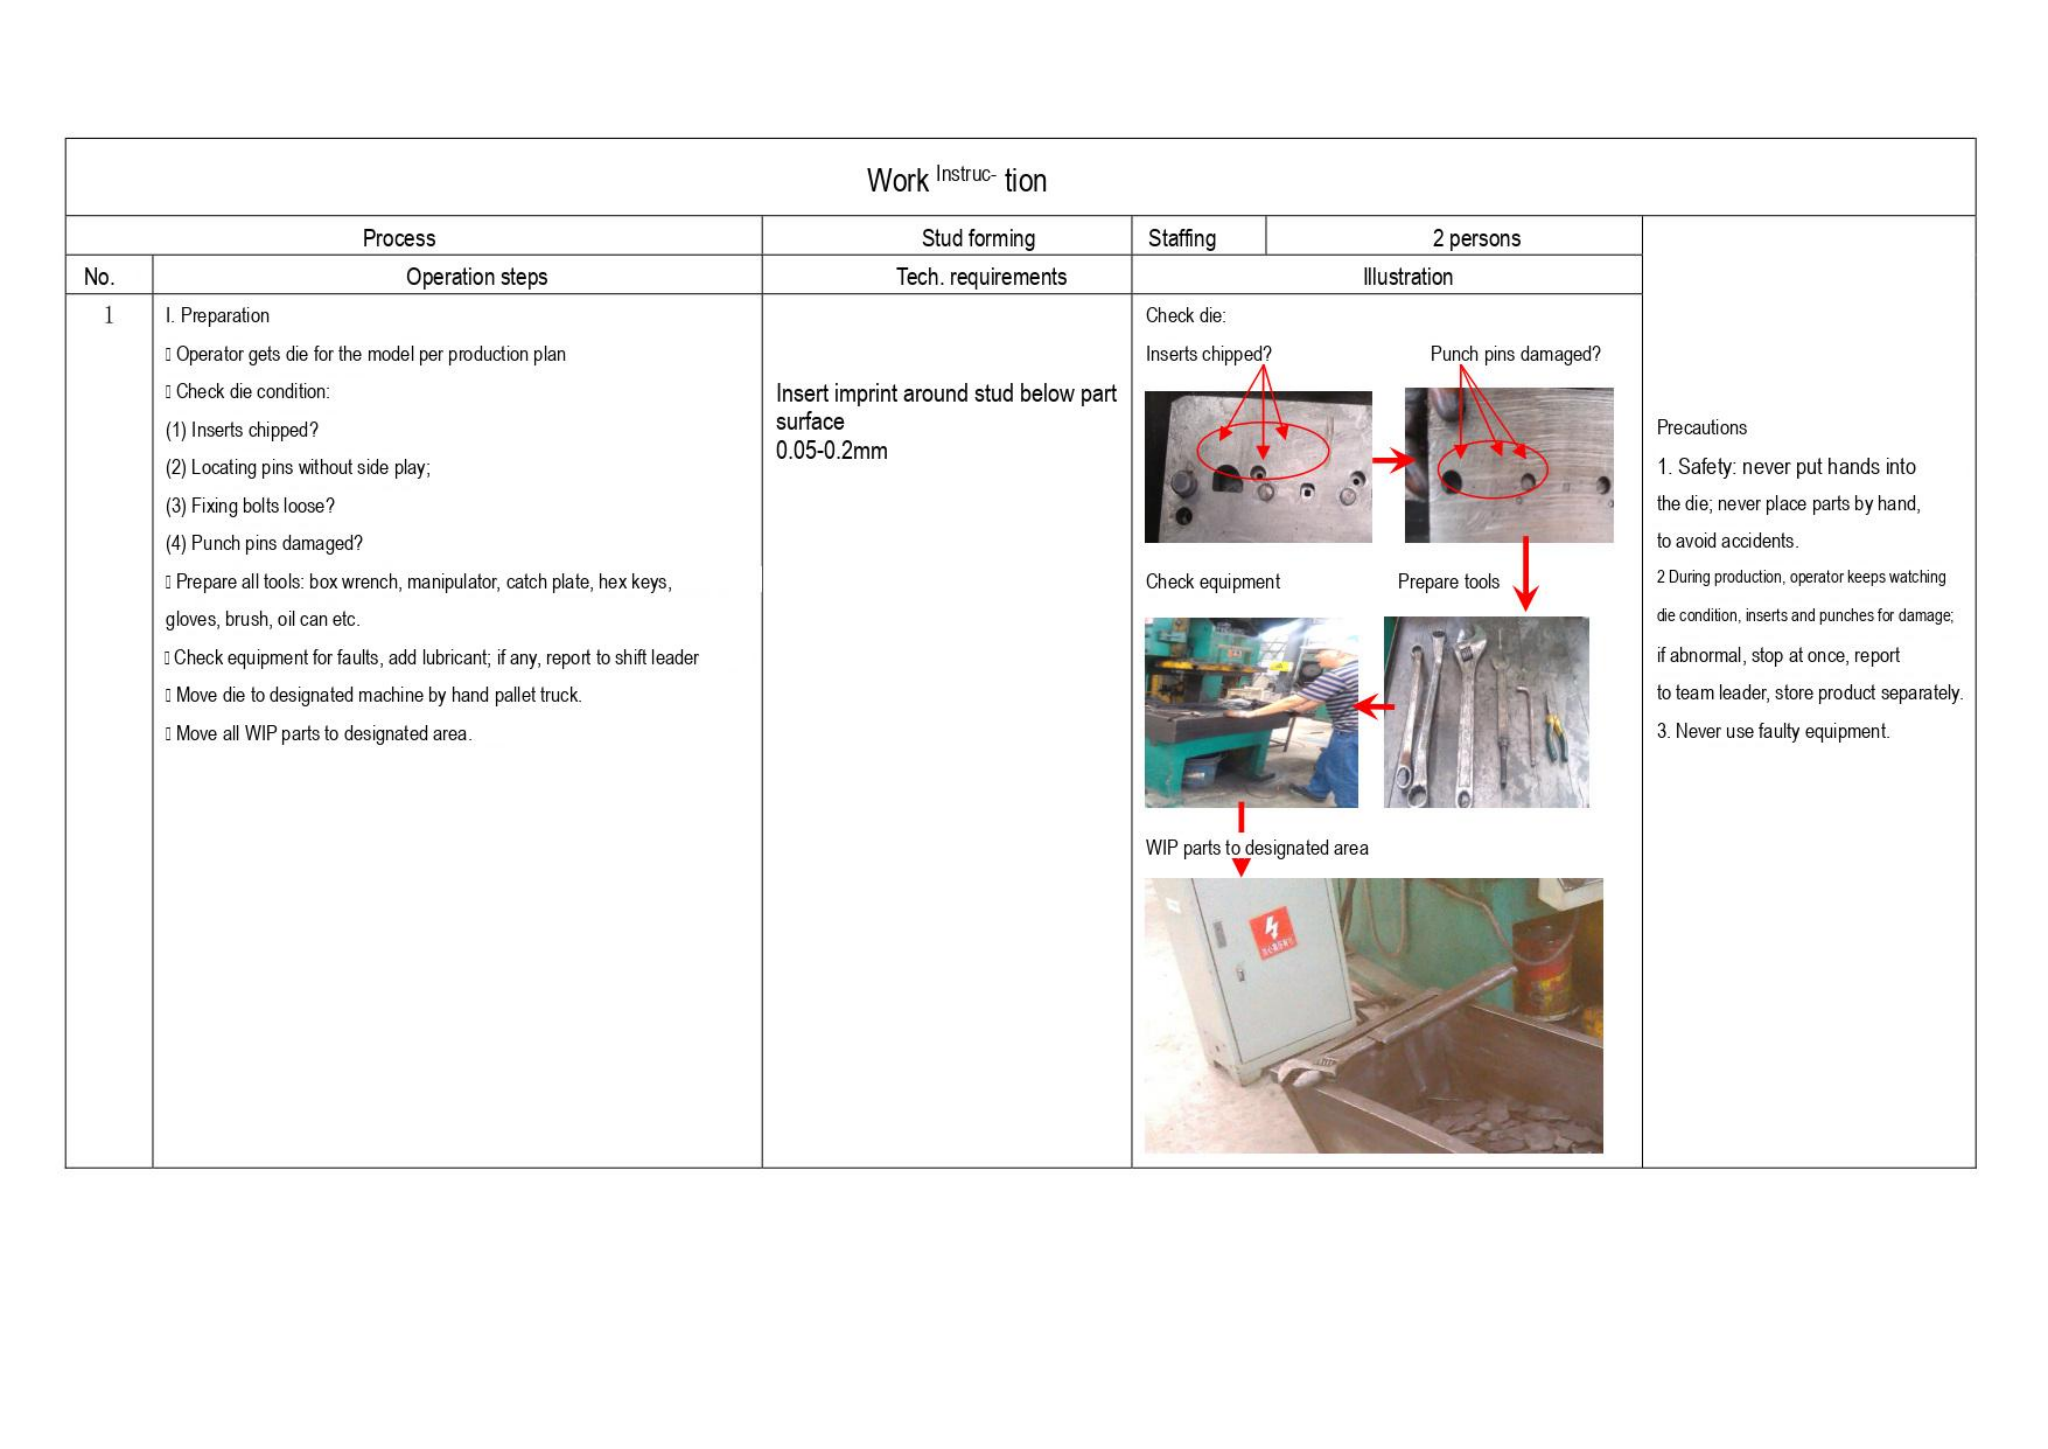# Work Instruc- tion

| Process | | Stud forming | Staffing | 2 persons | |
|---|---|---|---|---|---|
| **No.** | **Operation steps** | **Tech. requirements** | **Illustration** | | |
| 1 | I. Preparation<br>▯ Operator gets die for the model per production plan<br>▯ Check die condition:<br>(1) Inserts chipped?<br>(2) Locating pins without side play;<br>(3) Fixing bolts loose?<br>(4) Punch pins damaged?<br>▯ Prepare all tools: box wrench, manipulator, catch plate, hex keys, gloves, brush, oil can etc.<br>▯ Check equipment for faults, add lubricant; if any, report to shift leader<br>▯ Move die to designated machine by hand pallet truck.<br>▯ Move all WIP parts to designated area. | Insert imprint around stud below part surface<br>0.05-0.2mm | Check die:<br>Inserts chipped?<br>Punch pins damaged?<br>Check equipment<br>Prepare tools<br>WIP parts to designated area | | Precautions<br>1. Safety: never put hands into the die; never place parts by hand, to avoid accidents.<br>2 During production, operator keeps watching die condition, inserts and punches for damage; if abnormal, stop at once, report to team leader, store product separately.<br>3. Never use faulty equipment. |
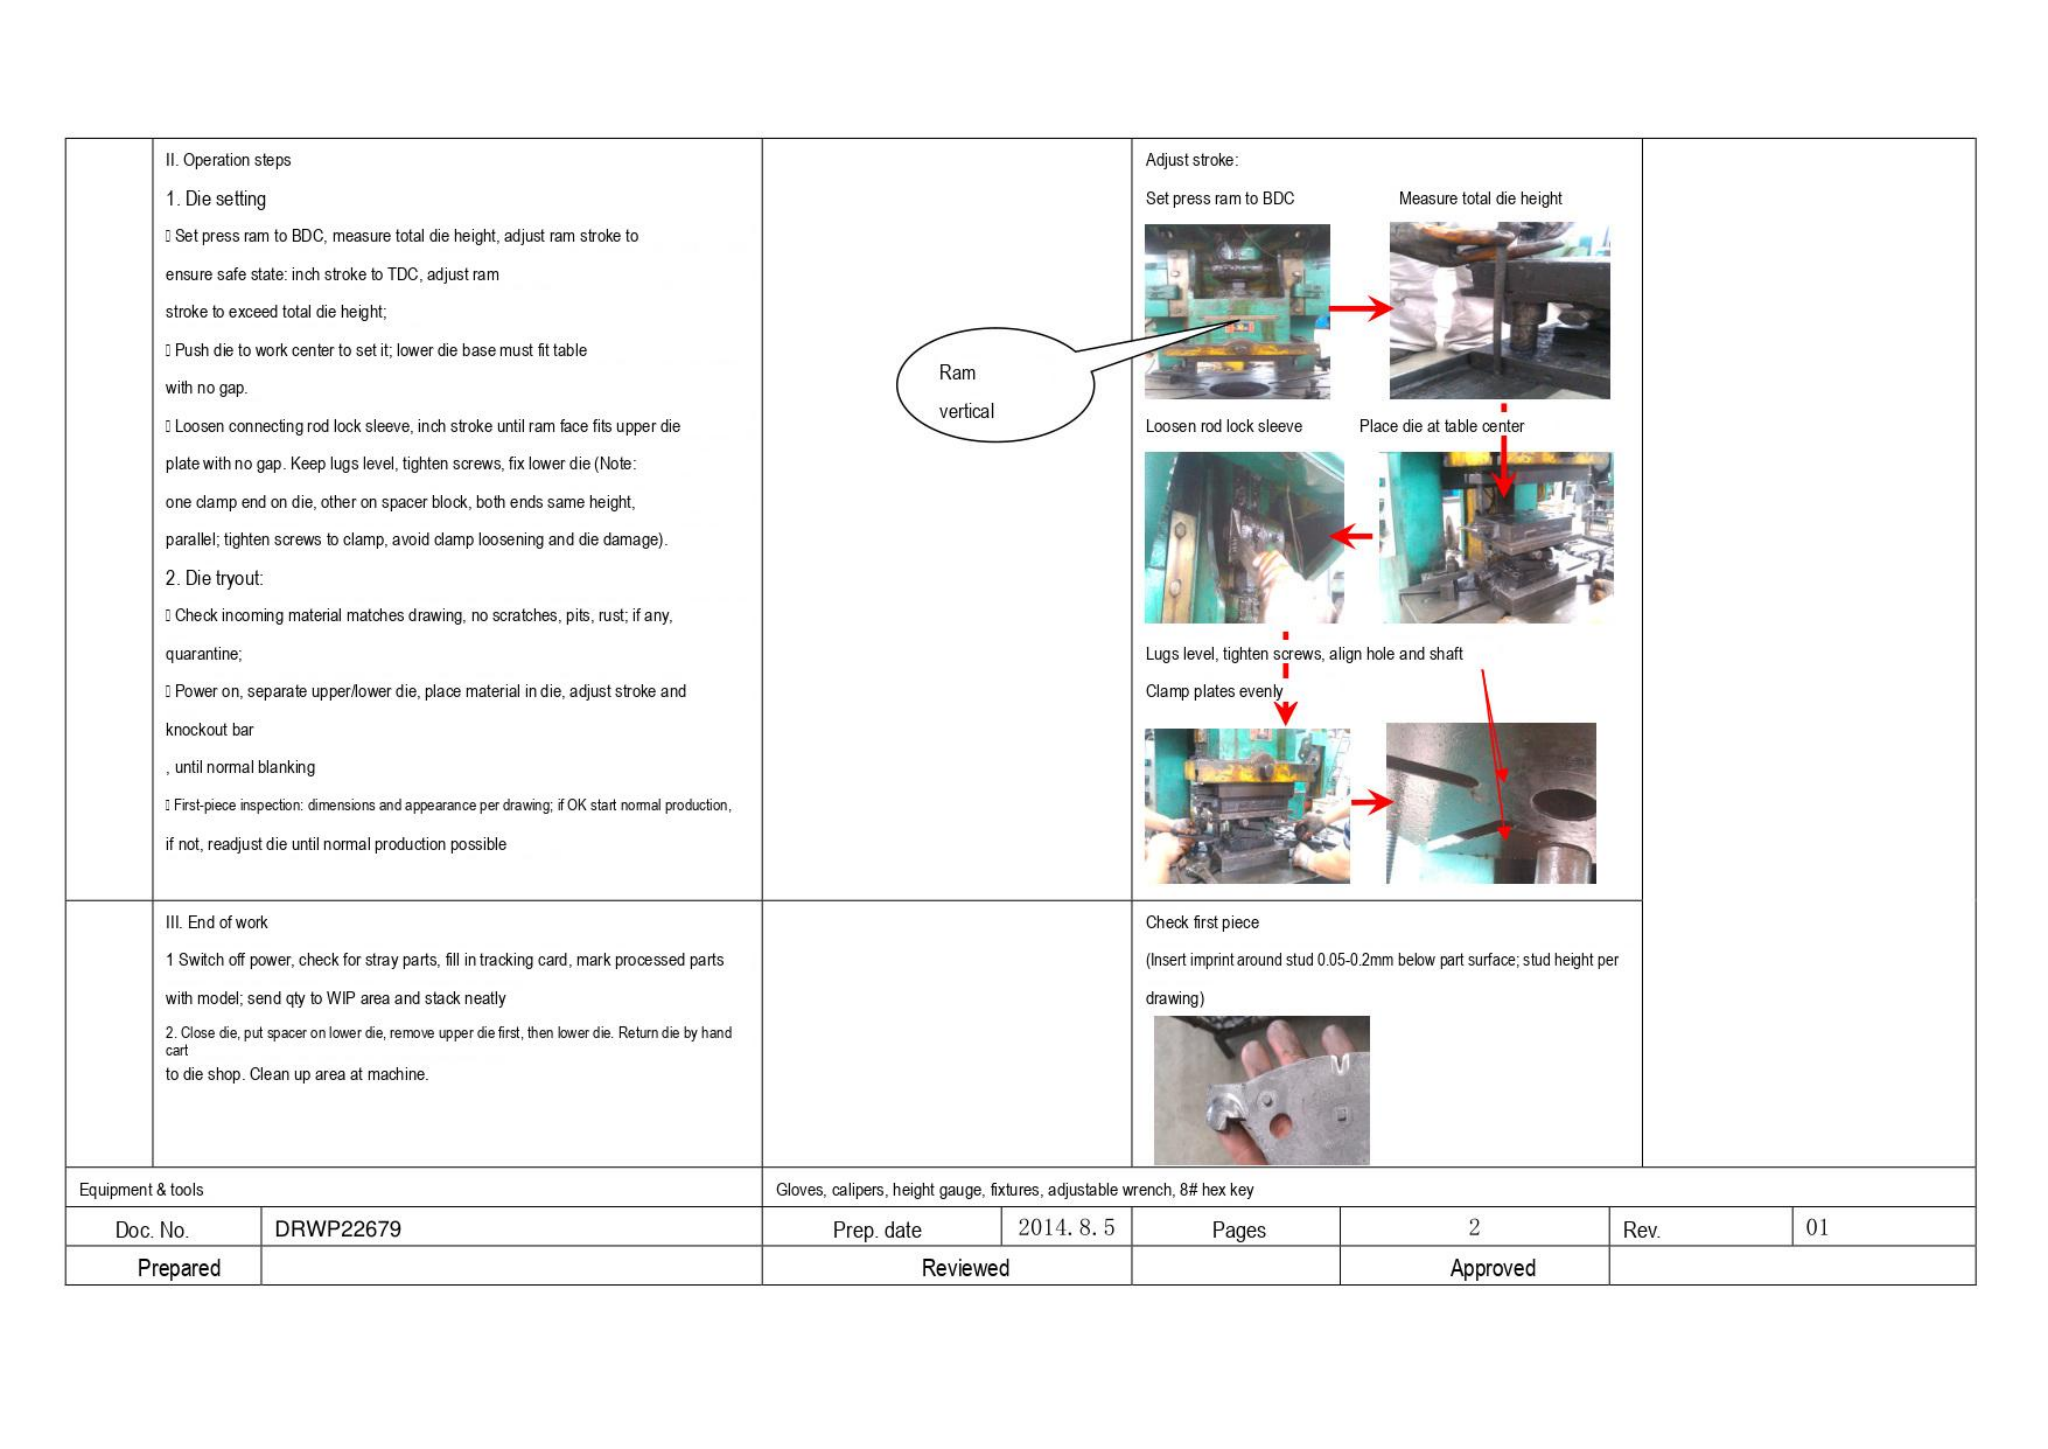| | | | | |
|---|---|---|---|---|
| | II. Operation steps<br>1. Die setting<br>Set press ram to BDC, measure total die height, adjust ram stroke to<br>ensure safe state: inch stroke to TDC, adjust ram<br>stroke to exceed total die height;<br>Push die to work center to set it; lower die base must fit table<br>with no gap.<br>Loosen connecting rod lock sleeve, inch stroke until ram face fits upper die<br>plate with no gap. Keep lugs level, tighten screws, fix lower die (Note:<br>one clamp end on die, other on spacer block, both ends same height,<br>parallel; tighten screws to clamp, avoid clamp loosening and die damage).<br>2. Die tryout:<br>Check incoming material matches drawing, no scratches, pits, rust; if any,<br>quarantine;<br>Power on, separate upper/lower die, place material in die, adjust stroke and<br>knockout bar<br>, until normal blanking<br>First-piece inspection: dimensions and appearance per drawing; if OK start normal production,<br>if not, readjust die until normal production possible | Ram<br>vertical | Adjust stroke:<br>Set press ram to BDC<br>Measure total die height<br>Loosen rod lock sleeve<br>Place die at table center<br>Lugs level, tighten screws, align hole and shaft<br>Clamp plates evenly | |
| | III. End of work<br>1 Switch off power, check for stray parts, fill in tracking card, mark processed parts<br>with model; send qty to WIP area and stack neatly<br>2. Close die, put spacer on lower die, remove upper die first, then lower die. Return die by hand cart<br>to die shop. Clean up area at machine. | | Check first piece<br>(Insert imprint around stud 0.05-0.2mm below part surface; stud height per<br>drawing) | |

| Equipment & tools | Gloves, calipers, height gauge, fixtures, adjustable wrench, 8# hex key |
|---|---|

| Doc. No. | DRWP22679 | Prep. date | 2014. 8. 5 | Pages | 2 | Rev. | 01 |
|---|---|---|---|---|---|---|---|
| Prepared | | Reviewed | | Approved | | | |